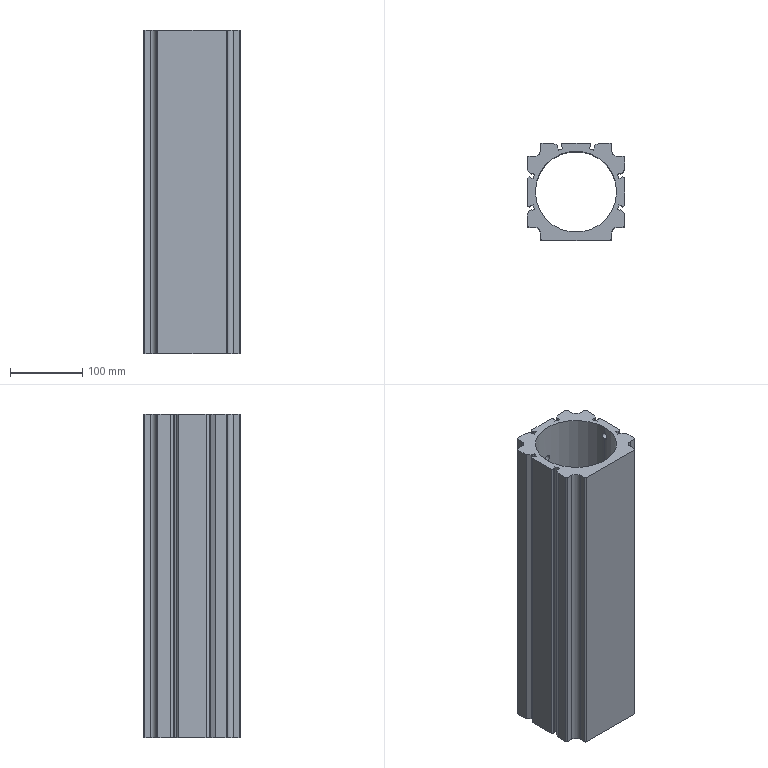Part | SolidWorks | features ICE 6, HoleWzd 5, Chamfer 3, CirPattern 3, Fillet 3, LPattern 2, MirrorPattern 2, Extrusion 1, MoveFace 1 | 1 solid | 118 faces | box 134 x 134 x 446.5 mm | volume 2883696 mm3 | plane 74 | cylinder 44 | commonest cylinder face diameters 9 x24 4 x8 8.8 x6 16 x4 112 x2